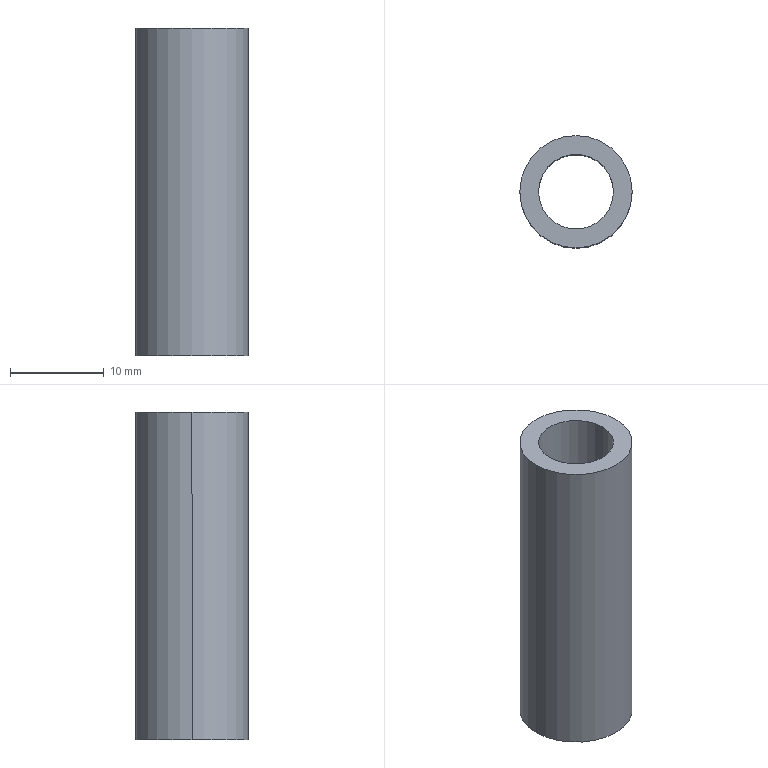Part | SolidWorks | features BaseBody 1 | 1 solid | 6 faces | box 12 x 12 x 35 mm | volume 2199 mm3 | cylinder 4 | plane 2 | commonest cylinder face diameters 8 x2 12 x2
STEP:
#1=CARTESIAN_POINT('',(-850.,-22.5,35.5));
#2=VERTEX_POINT('',#1);
#3=CARTESIAN_POINT('',(-838.,-22.5,35.5));
#4=VERTEX_POINT('',#3);
#5=CARTESIAN_POINT('',(-844.,-22.5,35.5));
#6=DIRECTION('',(0.,0.,-1.));
#7=DIRECTION('',(-1.,0.,0.));
#8=AXIS2_PLACEMENT_3D('',#5,#6,#7);
#9=CIRCLE('',#8,6.);
#10=EDGE_CURVE('',#2,#4,#9,.T.);
#11=ORIENTED_EDGE('',*,*,#10,.T.);
#12=CARTESIAN_POINT('',(-838.,-22.5,0.5));
#13=VERTEX_POINT('',#12);
#14=CARTESIAN_POINT('',(-838.,-22.5,0.5));
#15=DIRECTION('',(0.,0.,-1.));
#16=VECTOR('',#15,1000.);
#17=LINE('',#14,#16);
#18=EDGE_CURVE('',#4,#13,#17,.T.);
#19=ORIENTED_EDGE('',*,*,#18,.T.);
#20=CARTESIAN_POINT('',(-850.,-22.5,0.5));
#21=VERTEX_POINT('',#20);
#22=CARTESIAN_POINT('',(-844.,-22.5,0.5));
#23=DIRECTION('',(0.,0.,1.));
#24=DIRECTION('',(-1.,0.,0.));
#25=AXIS2_PLACEMENT_3D('',#22,#23,#24);
#26=CIRCLE('',#25,6.);
#27=EDGE_CURVE('',#13,#21,#26,.T.);
#28=ORIENTED_EDGE('',*,*,#27,.T.);
#29=CARTESIAN_POINT('',(-850.,-22.5,0.5));
#30=DIRECTION('',(0.,0.,-1.));
#31=VECTOR('',#30,1000.);
#32=LINE('',#29,#31);
#33=EDGE_CURVE('',#2,#21,#32,.T.);
#34=ORIENTED_EDGE('',*,*,#33,.F.);
#35=EDGE_LOOP('',(#11,#19,#28,#34));
#36=FACE_OUTER_BOUND('',#35,.T.);
#37=CARTESIAN_POINT('',(-844.,-22.5,0.5));
#38=DIRECTION('',(0.,0.,-1.));
#39=DIRECTION('',(-1.,0.,0.));
#40=AXIS2_PLACEMENT_3D('',#37,#38,#39);
#41=CYLINDRICAL_SURFACE('',#40,6.);
#42=ADVANCED_FACE('',(#36),#41,.T.);
#43=CARTESIAN_POINT('',(-840.,-22.5,35.5));
#44=VERTEX_POINT('',#43);
#45=CARTESIAN_POINT('',(-848.,-22.5,35.5));
#46=VERTEX_POINT('',#45);
#47=CARTESIAN_POINT('',(-844.,-22.5,35.5));
#48=DIRECTION('',(0.,0.,-1.));
#49=DIRECTION('',(-1.,0.,0.));
#50=AXIS2_PLACEMENT_3D('',#47,#48,#49);
#51=CIRCLE('',#50,4.);
#52=EDGE_CURVE('',#44,#46,#51,.T.);
#53=ORIENTED_EDGE('',*,*,#52,.F.);
#54=CARTESIAN_POINT('',(-840.,-22.5,0.5));
#55=VERTEX_POINT('',#54);
#56=CARTESIAN_POINT('',(-840.,-22.5,0.5));
#57=DIRECTION('',(0.,0.,-1.));
#58=VECTOR('',#57,1000.);
#59=LINE('',#56,#58);
#60=EDGE_CURVE('',#44,#55,#59,.T.);
#61=ORIENTED_EDGE('',*,*,#60,.T.);
#62=CARTESIAN_POINT('',(-848.,-22.5,0.5));
#63=VERTEX_POINT('',#62);
#64=CARTESIAN_POINT('',(-844.,-22.5,0.5));
#65=DIRECTION('',(0.,0.,1.));
#66=DIRECTION('',(-1.,0.,0.));
#67=AXIS2_PLACEMENT_3D('',#64,#65,#66);
#68=CIRCLE('',#67,4.);
#69=EDGE_CURVE('',#63,#55,#68,.T.);
#70=ORIENTED_EDGE('',*,*,#69,.F.);
#71=CARTESIAN_POINT('',(-848.,-22.5,0.5));
#72=DIRECTION('',(0.,0.,-1.));
#73=VECTOR('',#72,1000.);
#74=LINE('',#71,#73);
#75=EDGE_CURVE('',#46,#63,#74,.T.);
#76=ORIENTED_EDGE('',*,*,#75,.F.);
#77=EDGE_LOOP('',(#53,#61,#70,#76));
#78=FACE_OUTER_BOUND('',#77,.T.);
#79=CARTESIAN_POINT('',(-844.,-22.5,0.5));
#80=DIRECTION('',(0.,0.,-1.));
#81=DIRECTION('',(-1.,0.,0.));
#82=AXIS2_PLACEMENT_3D('',#79,#80,#81);
#83=CYLINDRICAL_SURFACE('',#82,4.);
#84=ADVANCED_FACE('',(#78),#83,.F.);
#85=ORIENTED_EDGE('',*,*,#18,.F.);
#86=CARTESIAN_POINT('',(-844.,-22.5,35.5));
#87=DIRECTION('',(0.,0.,-1.));
#88=DIRECTION('',(-1.,0.,0.));
#89=AXIS2_PLACEMENT_3D('',#86,#87,#88);
#90=CIRCLE('',#89,6.);
#91=EDGE_CURVE('',#4,#2,#90,.T.);
#92=ORIENTED_EDGE('',*,*,#91,.T.);
#93=ORIENTED_EDGE('',*,*,#33,.T.);
#94=CARTESIAN_POINT('',(-844.,-22.5,0.5));
#95=DIRECTION('',(0.,0.,1.));
#96=DIRECTION('',(-1.,0.,0.));
#97=AXIS2_PLACEMENT_3D('',#94,#95,#96);
#98=CIRCLE('',#97,6.);
#99=EDGE_CURVE('',#21,#13,#98,.T.);
#100=ORIENTED_EDGE('',*,*,#99,.T.);
#101=EDGE_LOOP('',(#85,#92,#93,#100));
#102=FACE_OUTER_BOUND('',#101,.T.);
#103=CARTESIAN_POINT('',(-844.,-22.5,0.5));
#104=DIRECTION('',(0.,0.,-1.));
#105=DIRECTION('',(-1.,0.,0.));
#106=AXIS2_PLACEMENT_3D('',#103,#104,#105);
#107=CYLINDRICAL_SURFACE('',#106,6.);
#108=ADVANCED_FACE('',(#102),#107,.T.);
#109=CARTESIAN_POINT('',(-844.,-22.5,35.5));
#110=DIRECTION('',(0.,0.,-1.));
#111=DIRECTION('',(-1.,0.,0.));
#112=AXIS2_PLACEMENT_3D('',#109,#110,#111);
#113=CIRCLE('',#112,4.);
#114=EDGE_CURVE('',#46,#44,#113,.T.);
#115=ORIENTED_EDGE('',*,*,#114,.T.);
#116=ORIENTED_EDGE('',*,*,#52,.T.);
#117=EDGE_LOOP('',(#115,#116));
#118=FACE_BOUND('',#117,.T.);
#119=ORIENTED_EDGE('',*,*,#10,.F.);
#120=ORIENTED_EDGE('',*,*,#91,.F.);
#121=EDGE_LOOP('',(#119,#120));
#122=FACE_OUTER_BOUND('',#121,.T.);
#123=CARTESIAN_POINT('',(-845.608,-22.5,35.5));
#124=DIRECTION('',(0.,0.,1.));
#125=DIRECTION('',(1.,0.,0.));
#126=AXIS2_PLACEMENT_3D('',#123,#124,#125);
#127=PLANE('',#126);
#128=ADVANCED_FACE('',(#118,#122),#127,.T.);
#129=ORIENTED_EDGE('',*,*,#69,.T.);
#130=CARTESIAN_POINT('',(-844.,-22.5,0.5));
#131=DIRECTION('',(0.,0.,1.));
#132=DIRECTION('',(-1.,0.,0.));
#133=AXIS2_PLACEMENT_3D('',#130,#131,#132);
#134=CIRCLE('',#133,4.);
#135=EDGE_CURVE('',#55,#63,#134,.T.);
#136=ORIENTED_EDGE('',*,*,#135,.T.);
#137=EDGE_LOOP('',(#129,#136));
#138=FACE_BOUND('',#137,.T.);
#139=ORIENTED_EDGE('',*,*,#99,.F.);
#140=ORIENTED_EDGE('',*,*,#27,.F.);
#141=EDGE_LOOP('',(#139,#140));
#142=FACE_OUTER_BOUND('',#141,.T.);
#143=CARTESIAN_POINT('',(-845.608,-22.5,0.5));
#144=DIRECTION('',(0.,0.,-1.));
#145=DIRECTION('',(0.,1.,0.));
#146=AXIS2_PLACEMENT_3D('',#143,#144,#145);
#147=PLANE('',#146);
#148=ADVANCED_FACE('',(#138,#142),#147,.T.);
#149=ORIENTED_EDGE('',*,*,#60,.F.);
#150=ORIENTED_EDGE('',*,*,#114,.F.);
#151=ORIENTED_EDGE('',*,*,#75,.T.);
#152=ORIENTED_EDGE('',*,*,#135,.F.);
#153=EDGE_LOOP('',(#149,#150,#151,#152));
#154=FACE_OUTER_BOUND('',#153,.T.);
#155=CARTESIAN_POINT('',(-844.,-22.5,0.5));
#156=DIRECTION('',(0.,0.,-1.));
#157=DIRECTION('',(-1.,0.,0.));
#158=AXIS2_PLACEMENT_3D('',#155,#156,#157);
#159=CYLINDRICAL_SURFACE('',#158,4.);
#160=ADVANCED_FACE('',(#154),#159,.F.);
#161=CLOSED_SHELL('',(#42,#84,#108,#128,#148,#160));
#162=MANIFOLD_SOLID_BREP('',#161);
#163=CARTESIAN_POINT('',(0.,0.,0.));
#164=DIRECTION('',(0.,0.,1.));
#165=DIRECTION('',(1.,0.,0.));
#166=AXIS2_PLACEMENT_3D('',#163,#164,#165);
#167=(LENGTH_UNIT()NAMED_UNIT(*)SI_UNIT(.MILLI.,.METRE.));
#168=UNCERTAINTY_MEASURE_WITH_UNIT(LENGTH_MEASURE(0.00001),#167,'','');
#169=(NAMED_UNIT(*)PLANE_ANGLE_UNIT()SI_UNIT($,.RADIAN.));
#170=(NAMED_UNIT(*)SI_UNIT($,.STERADIAN.)SOLID_ANGLE_UNIT());
#171=(GEOMETRIC_REPRESENTATION_CONTEXT(3)GLOBAL_UNCERTAINTY_ASSIGNED_CONTEXT((#168))GLOBAL_UNIT_ASSIGNED_CONTEXT((#167,#169,#170))REPRESENTATION_CONTEXT('',''));
#172=ADVANCED_BREP_SHAPE_REPRESENTATION('',(#162,#166),#171);